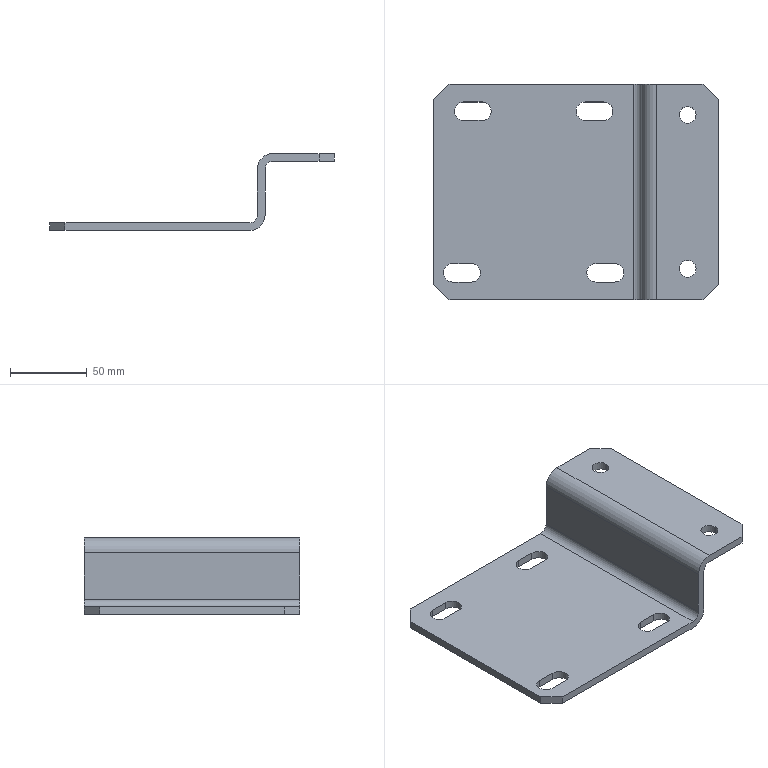Part | STEP file | VD-SYL0380DJ1006_1-8_VD-SYL0380 | 1 solid | 42 faces | box 185 x 140 x 50 mm | volume 149401 mm3 | plane 22 | cylinder 20 | commonest cylinder face diameters 12 x12 11 x4 10 x2 20 x2
STEP:
#1=CARTESIAN_POINT('',(-54.5,-58.5,-40.));
#2=VERTEX_POINT('',#1);
#3=CARTESIAN_POINT('',(-60.5,-52.5,-40.));
#4=VERTEX_POINT('',#3);
#5=CARTESIAN_POINT('',(-54.5,-52.5,-40.));
#6=DIRECTION('',(0.,0.,-1.));
#7=DIRECTION('',(0.,-1.,0.));
#8=AXIS2_PLACEMENT_3D('',#5,#6,#7);
#9=CIRCLE('',#8,6.);
#10=EDGE_CURVE('',#2,#4,#9,.T.);
#11=ORIENTED_EDGE('',*,*,#10,.F.);
#12=CARTESIAN_POINT('',(-54.5,-58.5,-45.));
#13=VERTEX_POINT('',#12);
#14=CARTESIAN_POINT('',(-54.5,-58.5,-40.));
#15=DIRECTION('',(0.,0.,-1.));
#16=VECTOR('',#15,1000.);
#17=LINE('',#14,#16);
#18=EDGE_CURVE('',#2,#13,#17,.T.);
#19=ORIENTED_EDGE('',*,*,#18,.T.);
#20=CARTESIAN_POINT('',(-60.5,-52.5,-45.));
#21=VERTEX_POINT('',#20);
#22=CARTESIAN_POINT('',(-54.5,-52.5,-45.));
#23=DIRECTION('',(0.,0.,1.));
#24=DIRECTION('',(-1.,0.,0.));
#25=AXIS2_PLACEMENT_3D('',#22,#23,#24);
#26=CIRCLE('',#25,6.);
#27=EDGE_CURVE('',#21,#13,#26,.T.);
#28=ORIENTED_EDGE('',*,*,#27,.F.);
#29=CARTESIAN_POINT('',(-60.5,-52.5,-45.));
#30=DIRECTION('',(0.,0.,1.));
#31=VECTOR('',#30,1000.);
#32=LINE('',#29,#31);
#33=EDGE_CURVE('',#21,#4,#32,.T.);
#34=ORIENTED_EDGE('',*,*,#33,.T.);
#35=EDGE_LOOP('',(#11,#19,#28,#34));
#36=FACE_OUTER_BOUND('',#35,.T.);
#37=CARTESIAN_POINT('',(-54.5,-52.5,-42.5));
#38=DIRECTION('',(0.,0.,-1.));
#39=DIRECTION('',(-1.,0.,0.));
#40=AXIS2_PLACEMENT_3D('',#37,#38,#39);
#41=CYLINDRICAL_SURFACE('',#40,6.);
#42=ADVANCED_FACE('',(#36),#41,.F.);
#43=ORIENTED_EDGE('',*,*,#33,.F.);
#44=CARTESIAN_POINT('',(-54.5,-46.5,-45.));
#45=VERTEX_POINT('',#44);
#46=CARTESIAN_POINT('',(-54.5,-52.5,-45.));
#47=DIRECTION('',(0.,0.,1.));
#48=DIRECTION('',(0.,1.,0.));
#49=AXIS2_PLACEMENT_3D('',#46,#47,#48);
#50=CIRCLE('',#49,6.);
#51=EDGE_CURVE('',#45,#21,#50,.T.);
#52=ORIENTED_EDGE('',*,*,#51,.F.);
#53=CARTESIAN_POINT('',(-54.5,-46.5,-40.));
#54=VERTEX_POINT('',#53);
#55=CARTESIAN_POINT('',(-54.5,-46.5,-45.));
#56=DIRECTION('',(0.,0.,1.));
#57=VECTOR('',#56,1000.);
#58=LINE('',#55,#57);
#59=EDGE_CURVE('',#45,#54,#58,.T.);
#60=ORIENTED_EDGE('',*,*,#59,.T.);
#61=CARTESIAN_POINT('',(-54.5,-52.5,-40.));
#62=DIRECTION('',(0.,0.,-1.));
#63=DIRECTION('',(-1.,0.,0.));
#64=AXIS2_PLACEMENT_3D('',#61,#62,#63);
#65=CIRCLE('',#64,6.);
#66=EDGE_CURVE('',#4,#54,#65,.T.);
#67=ORIENTED_EDGE('',*,*,#66,.F.);
#68=EDGE_LOOP('',(#43,#52,#60,#67));
#69=FACE_OUTER_BOUND('',#68,.T.);
#70=CARTESIAN_POINT('',(-54.5,-52.5,-42.5));
#71=DIRECTION('',(0.,0.,-1.));
#72=DIRECTION('',(-1.,0.,0.));
#73=AXIS2_PLACEMENT_3D('',#70,#71,#72);
#74=CYLINDRICAL_SURFACE('',#73,6.);
#75=ADVANCED_FACE('',(#69),#74,.F.);
#76=CARTESIAN_POINT('',(-42.5,-46.5,-45.));
#77=VERTEX_POINT('',#76);
#78=CARTESIAN_POINT('',(-54.5,-46.5,-45.));
#79=DIRECTION('',(1.,0.,0.));
#80=VECTOR('',#79,1000.);
#81=LINE('',#78,#80);
#82=EDGE_CURVE('',#45,#77,#81,.T.);
#83=ORIENTED_EDGE('',*,*,#82,.T.);
#84=CARTESIAN_POINT('',(-42.5,-46.5,-40.));
#85=VERTEX_POINT('',#84);
#86=CARTESIAN_POINT('',(-42.5,-46.5,-40.));
#87=DIRECTION('',(0.,0.,-1.));
#88=VECTOR('',#87,1000.);
#89=LINE('',#86,#88);
#90=EDGE_CURVE('',#85,#77,#89,.T.);
#91=ORIENTED_EDGE('',*,*,#90,.F.);
#92=CARTESIAN_POINT('',(-54.5,-46.5,-40.));
#93=DIRECTION('',(1.,0.,0.));
#94=VECTOR('',#93,1000.);
#95=LINE('',#92,#94);
#96=EDGE_CURVE('',#54,#85,#95,.T.);
#97=ORIENTED_EDGE('',*,*,#96,.F.);
#98=ORIENTED_EDGE('',*,*,#59,.F.);
#99=EDGE_LOOP('',(#83,#91,#97,#98));
#100=FACE_OUTER_BOUND('',#99,.T.);
#101=CARTESIAN_POINT('',(-48.5,-46.5,-42.5));
#102=DIRECTION('',(0.,-1.,0.));
#103=DIRECTION('',(0.,0.,-1.));
#104=AXIS2_PLACEMENT_3D('',#101,#102,#103);
#105=PLANE('',#104);
#106=ADVANCED_FACE('',(#100),#105,.T.);
#107=CARTESIAN_POINT('',(-42.5,-58.5,-40.));
#108=VERTEX_POINT('',#107);
#109=CARTESIAN_POINT('',(-42.5,-52.5,-40.));
#110=DIRECTION('',(0.,0.,-1.));
#111=DIRECTION('',(0.,1.,0.));
#112=AXIS2_PLACEMENT_3D('',#109,#110,#111);
#113=CIRCLE('',#112,6.);
#114=EDGE_CURVE('',#85,#108,#113,.T.);
#115=ORIENTED_EDGE('',*,*,#114,.F.);
#116=ORIENTED_EDGE('',*,*,#90,.T.);
#117=CARTESIAN_POINT('',(-42.5,-58.5,-45.));
#118=VERTEX_POINT('',#117);
#119=CARTESIAN_POINT('',(-42.5,-52.5,-45.));
#120=DIRECTION('',(0.,0.,1.));
#121=DIRECTION('',(1.,0.,0.));
#122=AXIS2_PLACEMENT_3D('',#119,#120,#121);
#123=CIRCLE('',#122,6.);
#124=EDGE_CURVE('',#118,#77,#123,.T.);
#125=ORIENTED_EDGE('',*,*,#124,.F.);
#126=CARTESIAN_POINT('',(-42.5,-58.5,-45.));
#127=DIRECTION('',(0.,0.,1.));
#128=VECTOR('',#127,1000.);
#129=LINE('',#126,#128);
#130=EDGE_CURVE('',#118,#108,#129,.T.);
#131=ORIENTED_EDGE('',*,*,#130,.T.);
#132=EDGE_LOOP('',(#115,#116,#125,#131));
#133=FACE_OUTER_BOUND('',#132,.T.);
#134=CARTESIAN_POINT('',(-42.5,-52.5,-42.5));
#135=DIRECTION('',(0.,0.,-1.));
#136=DIRECTION('',(-1.,0.,0.));
#137=AXIS2_PLACEMENT_3D('',#134,#135,#136);
#138=CYLINDRICAL_SURFACE('',#137,6.);
#139=ADVANCED_FACE('',(#133),#138,.F.);
#140=CARTESIAN_POINT('',(-42.5,-58.5,-45.));
#141=DIRECTION('',(-1.,0.,0.));
#142=VECTOR('',#141,1000.);
#143=LINE('',#140,#142);
#144=EDGE_CURVE('',#118,#13,#143,.T.);
#145=ORIENTED_EDGE('',*,*,#144,.T.);
#146=ORIENTED_EDGE('',*,*,#18,.F.);
#147=CARTESIAN_POINT('',(-42.5,-58.5,-40.));
#148=DIRECTION('',(-1.,0.,0.));
#149=VECTOR('',#148,1000.);
#150=LINE('',#147,#149);
#151=EDGE_CURVE('',#108,#2,#150,.T.);
#152=ORIENTED_EDGE('',*,*,#151,.F.);
#153=ORIENTED_EDGE('',*,*,#130,.F.);
#154=EDGE_LOOP('',(#145,#146,#152,#153));
#155=FACE_OUTER_BOUND('',#154,.T.);
#156=CARTESIAN_POINT('',(-48.5,-58.5,-42.5));
#157=DIRECTION('',(0.,1.,0.));
#158=DIRECTION('',(1.,0.,0.));
#159=AXIS2_PLACEMENT_3D('',#156,#157,#158);
#160=PLANE('',#159);
#161=ADVANCED_FACE('',(#155),#160,.T.);
#162=CARTESIAN_POINT('',(-147.5,-46.5,-45.));
#163=VERTEX_POINT('',#162);
#164=CARTESIAN_POINT('',(-135.5,-46.5,-45.));
#165=VERTEX_POINT('',#164);
#166=CARTESIAN_POINT('',(-147.5,-46.5,-45.));
#167=DIRECTION('',(1.,0.,0.));
#168=VECTOR('',#167,1000.);
#169=LINE('',#166,#168);
#170=EDGE_CURVE('',#163,#165,#169,.T.);
#171=ORIENTED_EDGE('',*,*,#170,.T.);
#172=CARTESIAN_POINT('',(-135.5,-46.5,-40.));
#173=VERTEX_POINT('',#172);
#174=CARTESIAN_POINT('',(-135.5,-46.5,-40.));
#175=DIRECTION('',(0.,0.,-1.));
#176=VECTOR('',#175,1000.);
#177=LINE('',#174,#176);
#178=EDGE_CURVE('',#173,#165,#177,.T.);
#179=ORIENTED_EDGE('',*,*,#178,.F.);
#180=CARTESIAN_POINT('',(-147.5,-46.5,-40.));
#181=VERTEX_POINT('',#180);
#182=CARTESIAN_POINT('',(-147.5,-46.5,-40.));
#183=DIRECTION('',(1.,0.,0.));
#184=VECTOR('',#183,1000.);
#185=LINE('',#182,#184);
#186=EDGE_CURVE('',#181,#173,#185,.T.);
#187=ORIENTED_EDGE('',*,*,#186,.F.);
#188=CARTESIAN_POINT('',(-147.5,-46.5,-45.));
#189=DIRECTION('',(0.,0.,1.));
#190=VECTOR('',#189,1000.);
#191=LINE('',#188,#190);
#192=EDGE_CURVE('',#163,#181,#191,.T.);
#193=ORIENTED_EDGE('',*,*,#192,.F.);
#194=EDGE_LOOP('',(#171,#179,#187,#193));
#195=FACE_OUTER_BOUND('',#194,.T.);
#196=CARTESIAN_POINT('',(-141.5,-46.5,-42.5));
#197=DIRECTION('',(0.,-1.,0.));
#198=DIRECTION('',(0.,0.,-1.));
#199=AXIS2_PLACEMENT_3D('',#196,#197,#198);
#200=PLANE('',#199);
#201=ADVANCED_FACE('',(#195),#200,.T.);
#202=CARTESIAN_POINT('',(-153.5,-52.5,-45.));
#203=VERTEX_POINT('',#202);
#204=CARTESIAN_POINT('',(-153.5,-52.5,-40.));
#205=VERTEX_POINT('',#204);
#206=CARTESIAN_POINT('',(-153.5,-52.5,-45.));
#207=DIRECTION('',(0.,0.,1.));
#208=VECTOR('',#207,1000.);
#209=LINE('',#206,#208);
#210=EDGE_CURVE('',#203,#205,#209,.T.);
#211=ORIENTED_EDGE('',*,*,#210,.F.);
#212=CARTESIAN_POINT('',(-147.5,-52.5,-45.));
#213=DIRECTION('',(0.,0.,1.));
#214=DIRECTION('',(0.,1.,0.));
#215=AXIS2_PLACEMENT_3D('',#212,#213,#214);
#216=CIRCLE('',#215,6.);
#217=EDGE_CURVE('',#163,#203,#216,.T.);
#218=ORIENTED_EDGE('',*,*,#217,.F.);
#219=ORIENTED_EDGE('',*,*,#192,.T.);
#220=CARTESIAN_POINT('',(-147.5,-52.5,-40.));
#221=DIRECTION('',(0.,0.,-1.));
#222=DIRECTION('',(-1.,0.,0.));
#223=AXIS2_PLACEMENT_3D('',#220,#221,#222);
#224=CIRCLE('',#223,6.);
#225=EDGE_CURVE('',#205,#181,#224,.T.);
#226=ORIENTED_EDGE('',*,*,#225,.F.);
#227=EDGE_LOOP('',(#211,#218,#219,#226));
#228=FACE_OUTER_BOUND('',#227,.T.);
#229=CARTESIAN_POINT('',(-147.5,-52.5,-42.5));
#230=DIRECTION('',(0.,0.,-1.));
#231=DIRECTION('',(-1.,0.,0.));
#232=AXIS2_PLACEMENT_3D('',#229,#230,#231);
#233=CYLINDRICAL_SURFACE('',#232,6.);
#234=ADVANCED_FACE('',(#228),#233,.F.);
#235=CARTESIAN_POINT('',(-147.5,-58.5,-40.));
#236=VERTEX_POINT('',#235);
#237=CARTESIAN_POINT('',(-147.5,-52.5,-40.));
#238=DIRECTION('',(0.,0.,-1.));
#239=DIRECTION('',(0.,-1.,0.));
#240=AXIS2_PLACEMENT_3D('',#237,#238,#239);
#241=CIRCLE('',#240,6.);
#242=EDGE_CURVE('',#236,#205,#241,.T.);
#243=ORIENTED_EDGE('',*,*,#242,.F.);
#244=CARTESIAN_POINT('',(-147.5,-58.5,-45.));
#245=VERTEX_POINT('',#244);
#246=CARTESIAN_POINT('',(-147.5,-58.5,-40.));
#247=DIRECTION('',(0.,0.,-1.));
#248=VECTOR('',#247,1000.);
#249=LINE('',#246,#248);
#250=EDGE_CURVE('',#236,#245,#249,.T.);
#251=ORIENTED_EDGE('',*,*,#250,.T.);
#252=CARTESIAN_POINT('',(-147.5,-52.5,-45.));
#253=DIRECTION('',(0.,0.,1.));
#254=DIRECTION('',(-1.,0.,0.));
#255=AXIS2_PLACEMENT_3D('',#252,#253,#254);
#256=CIRCLE('',#255,6.);
#257=EDGE_CURVE('',#203,#245,#256,.T.);
#258=ORIENTED_EDGE('',*,*,#257,.F.);
#259=ORIENTED_EDGE('',*,*,#210,.T.);
#260=EDGE_LOOP('',(#243,#251,#258,#259));
#261=FACE_OUTER_BOUND('',#260,.T.);
#262=CARTESIAN_POINT('',(-147.5,-52.5,-42.5));
#263=DIRECTION('',(0.,0.,-1.));
#264=DIRECTION('',(-1.,0.,0.));
#265=AXIS2_PLACEMENT_3D('',#262,#263,#264);
#266=CYLINDRICAL_SURFACE('',#265,6.);
#267=ADVANCED_FACE('',(#261),#266,.F.);
#268=CARTESIAN_POINT('',(-135.5,-58.5,-45.));
#269=VERTEX_POINT('',#268);
#270=CARTESIAN_POINT('',(-135.5,-58.5,-45.));
#271=DIRECTION('',(-1.,0.,0.));
#272=VECTOR('',#271,1000.);
#273=LINE('',#270,#272);
#274=EDGE_CURVE('',#269,#245,#273,.T.);
#275=ORIENTED_EDGE('',*,*,#274,.T.);
#276=ORIENTED_EDGE('',*,*,#250,.F.);
#277=CARTESIAN_POINT('',(-135.5,-58.5,-40.));
#278=VERTEX_POINT('',#277);
#279=CARTESIAN_POINT('',(-135.5,-58.5,-40.));
#280=DIRECTION('',(-1.,0.,0.));
#281=VECTOR('',#280,1000.);
#282=LINE('',#279,#281);
#283=EDGE_CURVE('',#278,#236,#282,.T.);
#284=ORIENTED_EDGE('',*,*,#283,.F.);
#285=CARTESIAN_POINT('',(-135.5,-58.5,-45.));
#286=DIRECTION('',(0.,0.,1.));
#287=VECTOR('',#286,1000.);
#288=LINE('',#285,#287);
#289=EDGE_CURVE('',#269,#278,#288,.T.);
#290=ORIENTED_EDGE('',*,*,#289,.F.);
#291=EDGE_LOOP('',(#275,#276,#284,#290));
#292=FACE_OUTER_BOUND('',#291,.T.);
#293=CARTESIAN_POINT('',(-141.5,-58.5,-42.5));
#294=DIRECTION('',(0.,1.,0.));
#295=DIRECTION('',(1.,0.,0.));
#296=AXIS2_PLACEMENT_3D('',#293,#294,#295);
#297=PLANE('',#296);
#298=ADVANCED_FACE('',(#292),#297,.T.);
#299=CARTESIAN_POINT('',(-135.5,-52.5,-40.));
#300=DIRECTION('',(0.,0.,-1.));
#301=DIRECTION('',(1.,0.,0.));
#302=AXIS2_PLACEMENT_3D('',#299,#300,#301);
#303=CIRCLE('',#302,6.);
#304=EDGE_CURVE('',#173,#278,#303,.T.);
#305=ORIENTED_EDGE('',*,*,#304,.F.);
#306=ORIENTED_EDGE('',*,*,#178,.T.);
#307=CARTESIAN_POINT('',(-135.5,-52.5,-45.));
#308=DIRECTION('',(0.,0.,1.));
#309=DIRECTION('',(0.,-1.,0.));
#310=AXIS2_PLACEMENT_3D('',#307,#308,#309);
#311=CIRCLE('',#310,6.);
#312=EDGE_CURVE('',#269,#165,#311,.T.);
#313=ORIENTED_EDGE('',*,*,#312,.F.);
#314=ORIENTED_EDGE('',*,*,#289,.T.);
#315=EDGE_LOOP('',(#305,#306,#313,#314));
#316=FACE_OUTER_BOUND('',#315,.T.);
#317=CARTESIAN_POINT('',(-135.5,-52.5,-42.5));
#318=DIRECTION('',(0.,0.,-1.));
#319=DIRECTION('',(-1.,0.,0.));
#320=AXIS2_PLACEMENT_3D('',#317,#318,#319);
#321=CYLINDRICAL_SURFACE('',#320,6.);
#322=ADVANCED_FACE('',(#316),#321,.F.);
#323=CARTESIAN_POINT('',(-61.5,46.5,-40.));
#324=VERTEX_POINT('',#323);
#325=CARTESIAN_POINT('',(-67.5,52.5,-40.));
#326=VERTEX_POINT('',#325);
#327=CARTESIAN_POINT('',(-61.5,52.5,-40.));
#328=DIRECTION('',(0.,0.,-1.));
#329=DIRECTION('',(0.,-1.,0.));
#330=AXIS2_PLACEMENT_3D('',#327,#328,#329);
#331=CIRCLE('',#330,6.);
#332=EDGE_CURVE('',#324,#326,#331,.T.);
#333=ORIENTED_EDGE('',*,*,#332,.F.);
#334=CARTESIAN_POINT('',(-61.5,46.5,-45.));
#335=VERTEX_POINT('',#334);
#336=CARTESIAN_POINT('',(-61.5,46.5,-40.));
#337=DIRECTION('',(0.,0.,-1.));
#338=VECTOR('',#337,1000.);
#339=LINE('',#336,#338);
#340=EDGE_CURVE('',#324,#335,#339,.T.);
#341=ORIENTED_EDGE('',*,*,#340,.T.);
#342=CARTESIAN_POINT('',(-67.5,52.5,-45.));
#343=VERTEX_POINT('',#342);
#344=CARTESIAN_POINT('',(-61.5,52.5,-45.));
#345=DIRECTION('',(0.,0.,1.));
#346=DIRECTION('',(-1.,0.,0.));
#347=AXIS2_PLACEMENT_3D('',#344,#345,#346);
#348=CIRCLE('',#347,6.);
#349=EDGE_CURVE('',#343,#335,#348,.T.);
#350=ORIENTED_EDGE('',*,*,#349,.F.);
#351=CARTESIAN_POINT('',(-67.5,52.5,-45.));
#352=DIRECTION('',(0.,0.,1.));
#353=VECTOR('',#352,1000.);
#354=LINE('',#351,#353);
#355=EDGE_CURVE('',#343,#326,#354,.T.);
#356=ORIENTED_EDGE('',*,*,#355,.T.);
#357=EDGE_LOOP('',(#333,#341,#350,#356));
#358=FACE_OUTER_BOUND('',#357,.T.);
#359=CARTESIAN_POINT('',(-61.5,52.5,-42.5));
#360=DIRECTION('',(0.,0.,-1.));
#361=DIRECTION('',(-1.,0.,0.));
#362=AXIS2_PLACEMENT_3D('',#359,#360,#361);
#363=CYLINDRICAL_SURFACE('',#362,6.);
#364=ADVANCED_FACE('',(#358),#363,.F.);
#365=ORIENTED_EDGE('',*,*,#355,.F.);
#366=CARTESIAN_POINT('',(-61.5,58.5,-45.));
#367=VERTEX_POINT('',#366);
#368=CARTESIAN_POINT('',(-61.5,52.5,-45.));
#369=DIRECTION('',(0.,0.,1.));
#370=DIRECTION('',(0.,1.,0.));
#371=AXIS2_PLACEMENT_3D('',#368,#369,#370);
#372=CIRCLE('',#371,6.);
#373=EDGE_CURVE('',#367,#343,#372,.T.);
#374=ORIENTED_EDGE('',*,*,#373,.F.);
#375=CARTESIAN_POINT('',(-61.5,58.5,-40.));
#376=VERTEX_POINT('',#375);
#377=CARTESIAN_POINT('',(-61.5,58.5,-45.));
#378=DIRECTION('',(0.,0.,1.));
#379=VECTOR('',#378,1000.);
#380=LINE('',#377,#379);
#381=EDGE_CURVE('',#367,#376,#380,.T.);
#382=ORIENTED_EDGE('',*,*,#381,.T.);
#383=CARTESIAN_POINT('',(-61.5,52.5,-40.));
#384=DIRECTION('',(0.,0.,-1.));
#385=DIRECTION('',(-1.,0.,0.));
#386=AXIS2_PLACEMENT_3D('',#383,#384,#385);
#387=CIRCLE('',#386,6.);
#388=EDGE_CURVE('',#326,#376,#387,.T.);
#389=ORIENTED_EDGE('',*,*,#388,.F.);
#390=EDGE_LOOP('',(#365,#374,#382,#389));
#391=FACE_OUTER_BOUND('',#390,.T.);
#392=CARTESIAN_POINT('',(-61.5,52.5,-42.5));
#393=DIRECTION('',(0.,0.,-1.));
#394=DIRECTION('',(-1.,0.,0.));
#395=AXIS2_PLACEMENT_3D('',#392,#393,#394);
#396=CYLINDRICAL_SURFACE('',#395,6.);
#397=ADVANCED_FACE('',(#391),#396,.F.);
#398=CARTESIAN_POINT('',(-49.5,58.5,-45.));
#399=VERTEX_POINT('',#398);
#400=CARTESIAN_POINT('',(-61.5,58.5,-45.));
#401=DIRECTION('',(1.,0.,0.));
#402=VECTOR('',#401,1000.);
#403=LINE('',#400,#402);
#404=EDGE_CURVE('',#367,#399,#403,.T.);
#405=ORIENTED_EDGE('',*,*,#404,.T.);
#406=CARTESIAN_POINT('',(-49.5,58.5,-40.));
#407=VERTEX_POINT('',#406);
#408=CARTESIAN_POINT('',(-49.5,58.5,-40.));
#409=DIRECTION('',(0.,0.,-1.));
#410=VECTOR('',#409,1000.);
#411=LINE('',#408,#410);
#412=EDGE_CURVE('',#407,#399,#411,.T.);
#413=ORIENTED_EDGE('',*,*,#412,.F.);
#414=CARTESIAN_POINT('',(-61.5,58.5,-40.));
#415=DIRECTION('',(1.,0.,0.));
#416=VECTOR('',#415,1000.);
#417=LINE('',#414,#416);
#418=EDGE_CURVE('',#376,#407,#417,.T.);
#419=ORIENTED_EDGE('',*,*,#418,.F.);
#420=ORIENTED_EDGE('',*,*,#381,.F.);
#421=EDGE_LOOP('',(#405,#413,#419,#420));
#422=FACE_OUTER_BOUND('',#421,.T.);
#423=CARTESIAN_POINT('',(-55.5,58.5,-42.5));
#424=DIRECTION('',(0.,-1.,0.));
#425=DIRECTION('',(0.,0.,-1.));
#426=AXIS2_PLACEMENT_3D('',#423,#424,#425);
#427=PLANE('',#426);
#428=ADVANCED_FACE('',(#422),#427,.T.);
#429=CARTESIAN_POINT('',(-49.5,46.5,-40.));
#430=VERTEX_POINT('',#429);
#431=CARTESIAN_POINT('',(-49.5,52.5,-40.));
#432=DIRECTION('',(0.,0.,-1.));
#433=DIRECTION('',(0.,1.,0.));
#434=AXIS2_PLACEMENT_3D('',#431,#432,#433);
#435=CIRCLE('',#434,6.);
#436=EDGE_CURVE('',#407,#430,#435,.T.);
#437=ORIENTED_EDGE('',*,*,#436,.F.);
#438=ORIENTED_EDGE('',*,*,#412,.T.);
#439=CARTESIAN_POINT('',(-49.5,46.5,-45.));
#440=VERTEX_POINT('',#439);
#441=CARTESIAN_POINT('',(-49.5,52.5,-45.));
#442=DIRECTION('',(0.,0.,1.));
#443=DIRECTION('',(1.,0.,0.));
#444=AXIS2_PLACEMENT_3D('',#441,#442,#443);
#445=CIRCLE('',#444,6.);
#446=EDGE_CURVE('',#440,#399,#445,.T.);
#447=ORIENTED_EDGE('',*,*,#446,.F.);
#448=CARTESIAN_POINT('',(-49.5,46.5,-45.));
#449=DIRECTION('',(0.,0.,1.));
#450=VECTOR('',#449,1000.);
#451=LINE('',#448,#450);
#452=EDGE_CURVE('',#440,#430,#451,.T.);
#453=ORIENTED_EDGE('',*,*,#452,.T.);
#454=EDGE_LOOP('',(#437,#438,#447,#453));
#455=FACE_OUTER_BOUND('',#454,.T.);
#456=CARTESIAN_POINT('',(-49.5,52.5,-42.5));
#457=DIRECTION('',(0.,0.,-1.));
#458=DIRECTION('',(-1.,0.,0.));
#459=AXIS2_PLACEMENT_3D('',#456,#457,#458);
#460=CYLINDRICAL_SURFACE('',#459,6.);
#461=ADVANCED_FACE('',(#455),#460,.F.);
#462=CARTESIAN_POINT('',(-49.5,46.5,-45.));
#463=DIRECTION('',(-1.,0.,0.));
#464=VECTOR('',#463,1000.);
#465=LINE('',#462,#464);
#466=EDGE_CURVE('',#440,#335,#465,.T.);
#467=ORIENTED_EDGE('',*,*,#466,.T.);
#468=ORIENTED_EDGE('',*,*,#340,.F.);
#469=CARTESIAN_POINT('',(-49.5,46.5,-40.));
#470=DIRECTION('',(-1.,0.,0.));
#471=VECTOR('',#470,1000.);
#472=LINE('',#469,#471);
#473=EDGE_CURVE('',#430,#324,#472,.T.);
#474=ORIENTED_EDGE('',*,*,#473,.F.);
#475=ORIENTED_EDGE('',*,*,#452,.F.);
#476=EDGE_LOOP('',(#467,#468,#474,#475));
#477=FACE_OUTER_BOUND('',#476,.T.);
#478=CARTESIAN_POINT('',(-55.5,46.5,-42.5));
#479=DIRECTION('',(0.,1.,0.));
#480=DIRECTION('',(1.,0.,0.));
#481=AXIS2_PLACEMENT_3D('',#478,#479,#480);
#482=PLANE('',#481);
#483=ADVANCED_FACE('',(#477),#482,.T.);
#484=CARTESIAN_POINT('',(-140.5,58.5,-45.));
#485=VERTEX_POINT('',#484);
#486=CARTESIAN_POINT('',(-128.5,58.5,-45.));
#487=VERTEX_POINT('',#486);
#488=CARTESIAN_POINT('',(-140.5,58.5,-45.));
#489=DIRECTION('',(1.,0.,0.));
#490=VECTOR('',#489,1000.);
#491=LINE('',#488,#490);
#492=EDGE_CURVE('',#485,#487,#491,.T.);
#493=ORIENTED_EDGE('',*,*,#492,.T.);
#494=CARTESIAN_POINT('',(-128.5,58.5,-40.));
#495=VERTEX_POINT('',#494);
#496=CARTESIAN_POINT('',(-128.5,58.5,-40.));
#497=DIRECTION('',(0.,0.,-1.));
#498=VECTOR('',#497,1000.);
#499=LINE('',#496,#498);
#500=EDGE_CURVE('',#495,#487,#499,.T.);
#501=ORIENTED_EDGE('',*,*,#500,.F.);
#502=CARTESIAN_POINT('',(-140.5,58.5,-40.));
#503=VERTEX_POINT('',#502);
#504=CARTESIAN_POINT('',(-140.5,58.5,-40.));
#505=DIRECTION('',(1.,0.,0.));
#506=VECTOR('',#505,1000.);
#507=LINE('',#504,#506);
#508=EDGE_CURVE('',#503,#495,#507,.T.);
#509=ORIENTED_EDGE('',*,*,#508,.F.);
#510=CARTESIAN_POINT('',(-140.5,58.5,-45.));
#511=DIRECTION('',(0.,0.,1.));
#512=VECTOR('',#511,1000.);
#513=LINE('',#510,#512);
#514=EDGE_CURVE('',#485,#503,#513,.T.);
#515=ORIENTED_EDGE('',*,*,#514,.F.);
#516=EDGE_LOOP('',(#493,#501,#509,#515));
#517=FACE_OUTER_BOUND('',#516,.T.);
#518=CARTESIAN_POINT('',(-134.5,58.5,-42.5));
#519=DIRECTION('',(0.,-1.,0.));
#520=DIRECTION('',(0.,0.,-1.));
#521=AXIS2_PLACEMENT_3D('',#518,#519,#520);
#522=PLANE('',#521);
#523=ADVANCED_FACE('',(#517),#522,.T.);
#524=CARTESIAN_POINT('',(-146.5,52.5,-45.));
#525=VERTEX_POINT('',#524);
#526=CARTESIAN_POINT('',(-146.5,52.5,-40.));
#527=VERTEX_POINT('',#526);
#528=CARTESIAN_POINT('',(-146.5,52.5,-45.));
#529=DIRECTION('',(0.,0.,1.));
#530=VECTOR('',#529,1000.);
#531=LINE('',#528,#530);
#532=EDGE_CURVE('',#525,#527,#531,.T.);
#533=ORIENTED_EDGE('',*,*,#532,.F.);
#534=CARTESIAN_POINT('',(-140.5,52.5,-45.));
#535=DIRECTION('',(0.,0.,1.));
#536=DIRECTION('',(0.,1.,0.));
#537=AXIS2_PLACEMENT_3D('',#534,#535,#536);
#538=CIRCLE('',#537,6.);
#539=EDGE_CURVE('',#485,#525,#538,.T.);
#540=ORIENTED_EDGE('',*,*,#539,.F.);
#541=ORIENTED_EDGE('',*,*,#514,.T.);
#542=CARTESIAN_POINT('',(-140.5,52.5,-40.));
#543=DIRECTION('',(0.,0.,-1.));
#544=DIRECTION('',(-1.,0.,0.));
#545=AXIS2_PLACEMENT_3D('',#542,#543,#544);
#546=CIRCLE('',#545,6.);
#547=EDGE_CURVE('',#527,#503,#546,.T.);
#548=ORIENTED_EDGE('',*,*,#547,.F.);
#549=EDGE_LOOP('',(#533,#540,#541,#548));
#550=FACE_OUTER_BOUND('',#549,.T.);
#551=CARTESIAN_POINT('',(-140.5,52.5,-42.5));
#552=DIRECTION('',(0.,0.,-1.));
#553=DIRECTION('',(-1.,0.,0.));
#554=AXIS2_PLACEMENT_3D('',#551,#552,#553);
#555=CYLINDRICAL_SURFACE('',#554,6.);
#556=ADVANCED_FACE('',(#550),#555,.F.);
#557=CARTESIAN_POINT('',(-140.5,46.5,-40.));
#558=VERTEX_POINT('',#557);
#559=CARTESIAN_POINT('',(-140.5,52.5,-40.));
#560=DIRECTION('',(0.,0.,-1.));
#561=DIRECTION('',(0.,-1.,0.));
#562=AXIS2_PLACEMENT_3D('',#559,#560,#561);
#563=CIRCLE('',#562,6.);
#564=EDGE_CURVE('',#558,#527,#563,.T.);
#565=ORIENTED_EDGE('',*,*,#564,.F.);
#566=CARTESIAN_POINT('',(-140.5,46.5,-45.));
#567=VERTEX_POINT('',#566);
#568=CARTESIAN_POINT('',(-140.5,46.5,-40.));
#569=DIRECTION('',(0.,0.,-1.));
#570=VECTOR('',#569,1000.);
#571=LINE('',#568,#570);
#572=EDGE_CURVE('',#558,#567,#571,.T.);
#573=ORIENTED_EDGE('',*,*,#572,.T.);
#574=CARTESIAN_POINT('',(-140.5,52.5,-45.));
#575=DIRECTION('',(0.,0.,1.));
#576=DIRECTION('',(-1.,0.,0.));
#577=AXIS2_PLACEMENT_3D('',#574,#575,#576);
#578=CIRCLE('',#577,6.);
#579=EDGE_CURVE('',#525,#567,#578,.T.);
#580=ORIENTED_EDGE('',*,*,#579,.F.);
#581=ORIENTED_EDGE('',*,*,#532,.T.);
#582=EDGE_LOOP('',(#565,#573,#580,#581));
#583=FACE_OUTER_BOUND('',#582,.T.);
#584=CARTESIAN_POINT('',(-140.5,52.5,-42.5));
#585=DIRECTION('',(0.,0.,-1.));
#586=DIRECTION('',(-1.,0.,0.));
#587=AXIS2_PLACEMENT_3D('',#584,#585,#586);
#588=CYLINDRICAL_SURFACE('',#587,6.);
#589=ADVANCED_FACE('',(#583),#588,.F.);
#590=CARTESIAN_POINT('',(-128.5,46.5,-45.));
#591=VERTEX_POINT('',#590);
#592=CARTESIAN_POINT('',(-128.5,46.5,-45.));
#593=DIRECTION('',(-1.,0.,0.));
#594=VECTOR('',#593,1000.);
#595=LINE('',#592,#594);
#596=EDGE_CURVE('',#591,#567,#595,.T.);
#597=ORIENTED_EDGE('',*,*,#596,.T.);
#598=ORIENTED_EDGE('',*,*,#572,.F.);
#599=CARTESIAN_POINT('',(-128.5,46.5,-40.));
#600=VERTEX_POINT('',#599);
#601=CARTESIAN_POINT('',(-128.5,46.5,-40.));
#602=DIRECTION('',(-1.,0.,0.));
#603=VECTOR('',#602,1000.);
#604=LINE('',#601,#603);
#605=EDGE_CURVE('',#600,#558,#604,.T.);
#606=ORIENTED_EDGE('',*,*,#605,.F.);
#607=CARTESIAN_POINT('',(-128.5,46.5,-45.));
#608=DIRECTION('',(0.,0.,1.));
#609=VECTOR('',#608,1000.);
#610=LINE('',#607,#609);
#611=EDGE_CURVE('',#591,#600,#610,.T.);
#612=ORIENTED_EDGE('',*,*,#611,.F.);
#613=EDGE_LOOP('',(#597,#598,#606,#612));
#614=FACE_OUTER_BOUND('',#613,.T.);
#615=CARTESIAN_POINT('',(-134.5,46.5,-42.5));
#616=DIRECTION('',(0.,1.,0.));
#617=DIRECTION('',(1.,0.,0.));
#618=AXIS2_PLACEMENT_3D('',#615,#616,#617);
#619=PLANE('',#618);
#620=ADVANCED_FACE('',(#614),#619,.T.);
#621=CARTESIAN_POINT('',(-128.5,52.5,-40.));
#622=DIRECTION('',(0.,0.,-1.));
#623=DIRECTION('',(1.,0.,0.));
#624=AXIS2_PLACEMENT_3D('',#621,#622,#623);
#625=CIRCLE('',#624,6.);
#626=EDGE_CURVE('',#495,#600,#625,.T.);
#627=ORIENTED_EDGE('',*,*,#626,.F.);
#628=ORIENTED_EDGE('',*,*,#500,.T.);
#629=CARTESIAN_POINT('',(-128.5,52.5,-45.));
#630=DIRECTION('',(0.,0.,1.));
#631=DIRECTION('',(0.,-1.,0.));
#632=AXIS2_PLACEMENT_3D('',#629,#630,#631);
#633=CIRCLE('',#632,6.);
#634=EDGE_CURVE('',#591,#487,#633,.T.);
#635=ORIENTED_EDGE('',*,*,#634,.F.);
#636=ORIENTED_EDGE('',*,*,#611,.T.);
#637=EDGE_LOOP('',(#627,#628,#635,#636));
#638=FACE_OUTER_BOUND('',#637,.T.);
#639=CARTESIAN_POINT('',(-128.5,52.5,-42.5));
#640=DIRECTION('',(0.,0.,-1.));
#641=DIRECTION('',(-1.,0.,0.));
#642=AXIS2_PLACEMENT_3D('',#639,#640,#641);
#643=CYLINDRICAL_SURFACE('',#642,6.);
#644=ADVANCED_FACE('',(#638),#643,.F.);
#645=CARTESIAN_POINT('',(-160.,60.,-45.));
#646=VERTEX_POINT('',#645);
#647=CARTESIAN_POINT('',(-150.,70.,-45.));
#648=VERTEX_POINT('',#647);
#649=CARTESIAN_POINT('',(-160.,60.,-45.));
#650=DIRECTION('',(0.7071,0.7071,0.));
#651=VECTOR('',#650,1000.);
#652=LINE('',#649,#651);
#653=EDGE_CURVE('',#646,#648,#652,.T.);
#654=ORIENTED_EDGE('',*,*,#653,.F.);
#655=CARTESIAN_POINT('',(-160.,60.,-40.));
#656=VERTEX_POINT('',#655);
#657=CARTESIAN_POINT('',(-160.,60.,-40.));
#658=DIRECTION('',(0.,0.,-1.));
#659=VECTOR('',#658,1000.);
#660=LINE('',#657,#659);
#661=EDGE_CURVE('',#656,#646,#660,.T.);
#662=ORIENTED_EDGE('',*,*,#661,.F.);
#663=CARTESIAN_POINT('',(-150.,70.,-40.));
#664=VERTEX_POINT('',#663);
#665=CARTESIAN_POINT('',(-150.,70.,-40.));
#666=DIRECTION('',(-0.7071,-0.7071,0.));
#667=VECTOR('',#666,1000.);
#668=LINE('',#665,#667);
#669=EDGE_CURVE('',#664,#656,#668,.T.);
#670=ORIENTED_EDGE('',*,*,#669,.F.);
#671=CARTESIAN_POINT('',(-150.,70.,-45.));
#672=DIRECTION('',(0.,0.,1.));
#673=VECTOR('',#672,1000.);
#674=LINE('',#671,#673);
#675=EDGE_CURVE('',#648,#664,#674,.T.);
#676=ORIENTED_EDGE('',*,*,#675,.F.);
#677=EDGE_LOOP('',(#654,#662,#670,#676));
#678=FACE_OUTER_BOUND('',#677,.T.);
#679=CARTESIAN_POINT('',(-155.,65.,-42.5));
#680=DIRECTION('',(-0.7071,0.7071,0.));
#681=DIRECTION('',(0.,0.,1.));
#682=AXIS2_PLACEMENT_3D('',#679,#680,#681);
#683=PLANE('',#682);
#684=ADVANCED_FACE('',(#678),#683,.T.);
#685=CARTESIAN_POINT('',(-30.,-70.,-45.));
#686=VERTEX_POINT('',#685);
#687=CARTESIAN_POINT('',(-30.,70.,-45.));
#688=VERTEX_POINT('',#687);
#689=CARTESIAN_POINT('',(-30.,-70.,-45.));
#690=DIRECTION('',(0.,1.,0.));
#691=VECTOR('',#690,1000.);
#692=LINE('',#689,#691);
#693=EDGE_CURVE('',#686,#688,#692,.T.);
#694=ORIENTED_EDGE('',*,*,#693,.T.);
#695=CARTESIAN_POINT('',(-20.,70.,-35.));
#696=VERTEX_POINT('',#695);
#697=CARTESIAN_POINT('',(-30.,70.,-35.));
#698=DIRECTION('',(0.,1.,0.));
#699=DIRECTION('',(1.,0.,0.));
#700=AXIS2_PLACEMENT_3D('',#697,#698,#699);
#701=CIRCLE('',#700,10.);
#702=EDGE_CURVE('',#696,#688,#701,.T.);
#703=ORIENTED_EDGE('',*,*,#702,.F.);
#704=CARTESIAN_POINT('',(-20.,-70.,-35.));
#705=VERTEX_POINT('',#704);
#706=CARTESIAN_POINT('',(-20.,70.,-35.));
#707=DIRECTION('',(0.,-1.,0.));
#708=VECTOR('',#707,1000.);
#709=LINE('',#706,#708);
#710=EDGE_CURVE('',#696,#705,#709,.T.);
#711=ORIENTED_EDGE('',*,*,#710,.T.);
#712=CARTESIAN_POINT('',(-30.,-70.,-35.));
#713=DIRECTION('',(0.,-1.,0.));
#714=DIRECTION('',(0.,0.,-1.));
#715=AXIS2_PLACEMENT_3D('',#712,#713,#714);
#716=CIRCLE('',#715,10.);
#717=EDGE_CURVE('',#686,#705,#716,.T.);
#718=ORIENTED_EDGE('',*,*,#717,.F.);
#719=EDGE_LOOP('',(#694,#703,#711,#718));
#720=FACE_OUTER_BOUND('',#719,.T.);
#721=CARTESIAN_POINT('',(-30.,70.,-35.));
#722=DIRECTION('',(0.,-1.,0.));
#723=DIRECTION('',(0.,0.,-1.));
#724=AXIS2_PLACEMENT_3D('',#721,#722,#723);
#725=CYLINDRICAL_SURFACE('',#724,10.);
#726=ADVANCED_FACE('',(#720),#725,.T.);
#727=CARTESIAN_POINT('',(-20.,-70.,-5.));
#728=VERTEX_POINT('',#727);
#729=CARTESIAN_POINT('',(-20.,70.,-5.));
#730=VERTEX_POINT('',#729);
#731=CARTESIAN_POINT('',(-20.,-70.,-5.));
#732=DIRECTION('',(0.,1.,0.));
#733=VECTOR('',#732,1000.);
#734=LINE('',#731,#733);
#735=EDGE_CURVE('',#728,#730,#734,.T.);
#736=ORIENTED_EDGE('',*,*,#735,.F.);
#737=CARTESIAN_POINT('',(-20.,-70.,-5.));
#738=DIRECTION('',(0.,0.,-1.));
#739=VECTOR('',#738,1000.);
#740=LINE('',#737,#739);
#741=EDGE_CURVE('',#728,#705,#740,.T.);
#742=ORIENTED_EDGE('',*,*,#741,.T.);
#743=ORIENTED_EDGE('',*,*,#710,.F.);
#744=CARTESIAN_POINT('',(-20.,70.,-35.));
#745=DIRECTION('',(0.,0.,1.));
#746=VECTOR('',#745,1000.);
#747=LINE('',#744,#746);
#748=EDGE_CURVE('',#696,#730,#747,.T.);
#749=ORIENTED_EDGE('',*,*,#748,.T.);
#750=EDGE_LOOP('',(#736,#742,#743,#749));
#751=FACE_OUTER_BOUND('',#750,.T.);
#752=CARTESIAN_POINT('',(-20.,70.,5.));
#753=DIRECTION('',(-1.,0.,0.));
#754=DIRECTION('',(0.,0.,1.));
#755=AXIS2_PLACEMENT_3D('',#752,#753,#754);
#756=PLANE('',#755);
#757=ADVANCED_FACE('',(#751),#756,.F.);
#758=CARTESIAN_POINT('',(10.5,50.,0.));
#759=VERTEX_POINT('',#758);
#760=CARTESIAN_POINT('',(10.5,50.,5.));
#761=VERTEX_POINT('',#760);
#762=CARTESIAN_POINT('',(10.5,50.,0.));
#763=DIRECTION('',(0.,0.,1.));
#764=VECTOR('',#763,1000.);
#765=LINE('',#762,#764);
#766=EDGE_CURVE('',#759,#761,#765,.T.);
#767=ORIENTED_EDGE('',*,*,#766,.F.);
#768=CARTESIAN_POINT('',(-0.5,50.,0.));
#769=VERTEX_POINT('',#768);
#770=CARTESIAN_POINT('',(5.,50.,0.));
#771=DIRECTION('',(0.,0.,1.));
#772=DIRECTION('',(-1.,0.,0.));
#773=AXIS2_PLACEMENT_3D('',#770,#771,#772);
#774=CIRCLE('',#773,5.5);
#775=EDGE_CURVE('',#769,#759,#774,.T.);
#776=ORIENTED_EDGE('',*,*,#775,.F.);
#777=CARTESIAN_POINT('',(-0.5,50.,5.));
#778=VERTEX_POINT('',#777);
#779=CARTESIAN_POINT('',(-0.5,50.,0.));
#780=DIRECTION('',(0.,0.,1.));
#781=VECTOR('',#780,1000.);
#782=LINE('',#779,#781);
#783=EDGE_CURVE('',#769,#778,#782,.T.);
#784=ORIENTED_EDGE('',*,*,#783,.T.);
#785=CARTESIAN_POINT('',(5.,50.,5.));
#786=DIRECTION('',(0.,0.,-1.));
#787=DIRECTION('',(1.,0.,0.));
#788=AXIS2_PLACEMENT_3D('',#785,#786,#787);
#789=CIRCLE('',#788,5.5);
#790=EDGE_CURVE('',#761,#778,#789,.T.);
#791=ORIENTED_EDGE('',*,*,#790,.F.);
#792=EDGE_LOOP('',(#767,#776,#784,#791));
#793=FACE_OUTER_BOUND('',#792,.T.);
#794=CARTESIAN_POINT('',(5.,50.,2.5));
#795=DIRECTION('',(0.,0.,-1.));
#796=DIRECTION('',(-1.,0.,0.));
#797=AXIS2_PLACEMENT_3D('',#794,#795,#796);
#798=CYLINDRICAL_SURFACE('',#797,5.5);
#799=ADVANCED_FACE('',(#793),#798,.F.);
#800=CARTESIAN_POINT('',(5.,50.,5.));
#801=DIRECTION('',(0.,0.,-1.));
#802=DIRECTION('',(-1.,0.,0.));
#803=AXIS2_PLACEMENT_3D('',#800,#801,#802);
#804=CIRCLE('',#803,5.5);
#805=EDGE_CURVE('',#778,#761,#804,.T.);
#806=ORIENTED_EDGE('',*,*,#805,.F.);
#807=ORIENTED_EDGE('',*,*,#783,.F.);
#808=CARTESIAN_POINT('',(5.,50.,0.));
#809=DIRECTION('',(0.,0.,1.));
#810=DIRECTION('',(1.,0.,0.));
#811=AXIS2_PLACEMENT_3D('',#808,#809,#810);
#812=CIRCLE('',#811,5.5);
#813=EDGE_CURVE('',#759,#769,#812,.T.);
#814=ORIENTED_EDGE('',*,*,#813,.F.);
#815=ORIENTED_EDGE('',*,*,#766,.T.);
#816=EDGE_LOOP('',(#806,#807,#814,#815));
#817=FACE_OUTER_BOUND('',#816,.T.);
#818=CARTESIAN_POINT('',(5.,50.,2.5));
#819=DIRECTION('',(0.,0.,-1.));
#820=DIRECTION('',(-1.,0.,0.));
#821=AXIS2_PLACEMENT_3D('',#818,#819,#820);
#822=CYLINDRICAL_SURFACE('',#821,5.5);
#823=ADVANCED_FACE('',(#817),#822,.F.);
#824=CARTESIAN_POINT('',(10.5,-50.,0.));
#825=VERTEX_POINT('',#824);
#826=CARTESIAN_POINT('',(10.5,-50.,5.));
#827=VERTEX_POINT('',#826);
#828=CARTESIAN_POINT('',(10.5,-50.,0.));
#829=DIRECTION('',(0.,0.,1.));
#830=VECTOR('',#829,1000.);
#831=LINE('',#828,#830);
#832=EDGE_CURVE('',#825,#827,#831,.T.);
#833=ORIENTED_EDGE('',*,*,#832,.F.);
#834=CARTESIAN_POINT('',(-0.5,-50.,0.));
#835=VERTEX_POINT('',#834);
#836=CARTESIAN_POINT('',(5.,-50.,0.));
#837=DIRECTION('',(0.,0.,1.));
#838=DIRECTION('',(-1.,0.,0.));
#839=AXIS2_PLACEMENT_3D('',#836,#837,#838);
#840=CIRCLE('',#839,5.5);
#841=EDGE_CURVE('',#835,#825,#840,.T.);
#842=ORIENTED_EDGE('',*,*,#841,.F.);
#843=CARTESIAN_POINT('',(-0.5,-50.,5.));
#844=VERTEX_POINT('',#843);
#845=CARTESIAN_POINT('',(-0.5,-50.,0.));
#846=DIRECTION('',(0.,0.,1.));
#847=VECTOR('',#846,1000.);
#848=LINE('',#845,#847);
#849=EDGE_CURVE('',#835,#844,#848,.T.);
#850=ORIENTED_EDGE('',*,*,#849,.T.);
#851=CARTESIAN_POINT('',(5.,-50.,5.));
#852=DIRECTION('',(0.,0.,-1.));
#853=DIRECTION('',(1.,0.,0.));
#854=AXIS2_PLACEMENT_3D('',#851,#852,#853);
#855=CIRCLE('',#854,5.5);
#856=EDGE_CURVE('',#827,#844,#855,.T.);
#857=ORIENTED_EDGE('',*,*,#856,.F.);
#858=EDGE_LOOP('',(#833,#842,#850,#857));
#859=FACE_OUTER_BOUND('',#858,.T.);
#860=CARTESIAN_POINT('',(5.,-50.,2.5));
#861=DIRECTION('',(0.,0.,-1.));
#862=DIRECTION('',(-1.,0.,0.));
#863=AXIS2_PLACEMENT_3D('',#860,#861,#862);
#864=CYLINDRICAL_SURFACE('',#863,5.5);
#865=ADVANCED_FACE('',(#859),#864,.F.);
#866=CARTESIAN_POINT('',(5.,-50.,5.));
#867=DIRECTION('',(0.,0.,-1.));
#868=DIRECTION('',(-1.,0.,0.));
#869=AXIS2_PLACEMENT_3D('',#866,#867,#868);
#870=CIRCLE('',#869,5.5);
#871=EDGE_CURVE('',#844,#827,#870,.T.);
#872=ORIENTED_EDGE('',*,*,#871,.F.);
#873=ORIENTED_EDGE('',*,*,#849,.F.);
#874=CARTESIAN_POINT('',(5.,-50.,0.));
#875=DIRECTION('',(0.,0.,1.));
#876=DIRECTION('',(1.,0.,0.));
#877=AXIS2_PLACEMENT_3D('',#874,#875,#876);
#878=CIRCLE('',#877,5.5);
#879=EDGE_CURVE('',#825,#835,#878,.T.);
#880=ORIENTED_EDGE('',*,*,#879,.F.);
#881=ORIENTED_EDGE('',*,*,#832,.T.);
#882=EDGE_LOOP('',(#872,#873,#880,#881));
#883=FACE_OUTER_BOUND('',#882,.T.);
#884=CARTESIAN_POINT('',(5.,-50.,2.5));
#885=DIRECTION('',(0.,0.,-1.));
#886=DIRECTION('',(-1.,0.,0.));
#887=AXIS2_PLACEMENT_3D('',#884,#885,#886);
#888=CYLINDRICAL_SURFACE('',#887,5.5);
#889=ADVANCED_FACE('',(#883),#888,.F.);
#890=CARTESIAN_POINT('',(25.,-60.,0.));
#891=VERTEX_POINT('',#890);
#892=CARTESIAN_POINT('',(15.,-70.,0.));
#893=VERTEX_POINT('',#892);
#894=CARTESIAN_POINT('',(25.,-60.,0.));
#895=DIRECTION('',(-0.7071,-0.7071,0.));
#896=VECTOR('',#895,1000.);
#897=LINE('',#894,#896);
#898=EDGE_CURVE('',#891,#893,#897,.T.);
#899=ORIENTED_EDGE('',*,*,#898,.F.);
#900=CARTESIAN_POINT('',(25.,-60.,5.));
#901=VERTEX_POINT('',#900);
#902=CARTESIAN_POINT('',(25.,-60.,5.));
#903=DIRECTION('',(0.,0.,-1.));
#904=VECTOR('',#903,1000.);
#905=LINE('',#902,#904);
#906=EDGE_CURVE('',#901,#891,#905,.T.);
#907=ORIENTED_EDGE('',*,*,#906,.F.);
#908=CARTESIAN_POINT('',(15.,-70.,5.));
#909=VERTEX_POINT('',#908);
#910=CARTESIAN_POINT('',(15.,-70.,5.));
#911=DIRECTION('',(0.7071,0.7071,0.));
#912=VECTOR('',#911,1000.);
#913=LINE('',#910,#912);
#914=EDGE_CURVE('',#909,#901,#913,.T.);
#915=ORIENTED_EDGE('',*,*,#914,.F.);
#916=CARTESIAN_POINT('',(15.,-70.,0.));
#917=DIRECTION('',(0.,0.,1.));
#918=VECTOR('',#917,1000.);
#919=LINE('',#916,#918);
#920=EDGE_CURVE('',#893,#909,#919,.T.);
#921=ORIENTED_EDGE('',*,*,#920,.F.);
#922=EDGE_LOOP('',(#899,#907,#915,#921));
#923=FACE_OUTER_BOUND('',#922,.T.);
#924=CARTESIAN_POINT('',(20.,-65.,2.5));
#925=DIRECTION('',(0.7071,-0.7071,0.));
#926=DIRECTION('',(0.,0.,-1.));
#927=AXIS2_PLACEMENT_3D('',#924,#925,#926);
#928=PLANE('',#927);
#929=ADVANCED_FACE('',(#923),#928,.T.);
#930=ORIENTED_EDGE('',*,*,#790,.T.);
#931=ORIENTED_EDGE('',*,*,#805,.T.);
#932=EDGE_LOOP('',(#930,#931));
#933=FACE_BOUND('',#932,.T.);
#934=ORIENTED_EDGE('',*,*,#856,.T.);
#935=ORIENTED_EDGE('',*,*,#871,.T.);
#936=EDGE_LOOP('',(#934,#935));
#937=FACE_BOUND('',#936,.T.);
#938=ORIENTED_EDGE('',*,*,#914,.T.);
#939=CARTESIAN_POINT('',(25.,60.,5.));
#940=VERTEX_POINT('',#939);
#941=CARTESIAN_POINT('',(25.,60.,5.));
#942=DIRECTION('',(0.,-1.,0.));
#943=VECTOR('',#942,1000.);
#944=LINE('',#941,#943);
#945=EDGE_CURVE('',#940,#901,#944,.T.);
#946=ORIENTED_EDGE('',*,*,#945,.F.);
#947=CARTESIAN_POINT('',(15.,70.,5.));
#948=VERTEX_POINT('',#947);
#949=CARTESIAN_POINT('',(25.,60.,5.));
#950=DIRECTION('',(-0.7071,0.7071,0.));
#951=VECTOR('',#950,1000.);
#952=LINE('',#949,#951);
#953=EDGE_CURVE('',#940,#948,#952,.T.);
#954=ORIENTED_EDGE('',*,*,#953,.T.);
#955=CARTESIAN_POINT('',(-15.,70.,5.));
#956=VERTEX_POINT('',#955);
#957=CARTESIAN_POINT('',(-15.,70.,5.));
#958=DIRECTION('',(1.,0.,0.));
#959=VECTOR('',#958,1000.);
#960=LINE('',#957,#959);
#961=EDGE_CURVE('',#956,#948,#960,.T.);
#962=ORIENTED_EDGE('',*,*,#961,.F.);
#963=CARTESIAN_POINT('',(-15.,-70.,5.));
#964=VERTEX_POINT('',#963);
#965=CARTESIAN_POINT('',(-15.,-70.,5.));
#966=DIRECTION('',(0.,1.,0.));
#967=VECTOR('',#966,1000.);
#968=LINE('',#965,#967);
#969=EDGE_CURVE('',#964,#956,#968,.T.);
#970=ORIENTED_EDGE('',*,*,#969,.F.);
#971=CARTESIAN_POINT('',(15.,-70.,5.));
#972=DIRECTION('',(-1.,0.,0.));
#973=VECTOR('',#972,1000.);
#974=LINE('',#971,#973);
#975=EDGE_CURVE('',#909,#964,#974,.T.);
#976=ORIENTED_EDGE('',*,*,#975,.F.);
#977=EDGE_LOOP('',(#938,#946,#954,#962,#970,#976));
#978=FACE_OUTER_BOUND('',#977,.T.);
#979=CARTESIAN_POINT('',(0.,0.,5.));
#980=DIRECTION('',(0.,0.,1.));
#981=DIRECTION('',(1.,0.,0.));
#982=AXIS2_PLACEMENT_3D('',#979,#980,#981);
#983=PLANE('',#982);
#984=ADVANCED_FACE('',(#933,#937,#978),#983,.T.);
#985=CARTESIAN_POINT('',(-25.,70.,-5.));
#986=VERTEX_POINT('',#985);
#987=CARTESIAN_POINT('',(-25.,-70.,-5.));
#988=VERTEX_POINT('',#987);
#989=CARTESIAN_POINT('',(-25.,70.,-5.));
#990=DIRECTION('',(0.,-1.,0.));
#991=VECTOR('',#990,1000.);
#992=LINE('',#989,#991);
#993=EDGE_CURVE('',#986,#988,#992,.T.);
#994=ORIENTED_EDGE('',*,*,#993,.T.);
#995=CARTESIAN_POINT('',(-15.,-70.,-5.));
#996=DIRECTION('',(0.,-1.,0.));
#997=DIRECTION('',(0.,0.,1.));
#998=AXIS2_PLACEMENT_3D('',#995,#996,#997);
#999=CIRCLE('',#998,10.);
#1000=EDGE_CURVE('',#964,#988,#999,.T.);
#1001=ORIENTED_EDGE('',*,*,#1000,.F.);
#1002=ORIENTED_EDGE('',*,*,#969,.T.);
#1003=CARTESIAN_POINT('',(-15.,70.,-5.));
#1004=DIRECTION('',(0.,1.,0.));
#1005=DIRECTION('',(-1.,0.,0.));
#1006=AXIS2_PLACEMENT_3D('',#1003,#1004,#1005);
#1007=CIRCLE('',#1006,10.);
#1008=EDGE_CURVE('',#986,#956,#1007,.T.);
#1009=ORIENTED_EDGE('',*,*,#1008,.F.);
#1010=EDGE_LOOP('',(#994,#1001,#1002,#1009));
#1011=FACE_OUTER_BOUND('',#1010,.T.);
#1012=CARTESIAN_POINT('',(-15.,-70.,-5.));
#1013=DIRECTION('',(0.,1.,0.));
#1014=DIRECTION('',(0.,0.,1.));
#1015=AXIS2_PLACEMENT_3D('',#1012,#1013,#1014);
#1016=CYLINDRICAL_SURFACE('',#1015,10.);
#1017=ADVANCED_FACE('',(#1011),#1016,.T.);
#1018=CARTESIAN_POINT('',(-25.,70.,-35.));
#1019=VERTEX_POINT('',#1018);
#1020=CARTESIAN_POINT('',(-25.,70.,-5.));
#1021=DIRECTION('',(0.,0.,-1.));
#1022=VECTOR('',#1021,1000.);
#1023=LINE('',#1020,#1022);
#1024=EDGE_CURVE('',#986,#1019,#1023,.T.);
#1025=ORIENTED_EDGE('',*,*,#1024,.T.);
#1026=CARTESIAN_POINT('',(-25.,-70.,-35.));
#1027=VERTEX_POINT('',#1026);
#1028=CARTESIAN_POINT('',(-25.,-70.,-35.));
#1029=DIRECTION('',(0.,1.,0.));
#1030=VECTOR('',#1029,1000.);
#1031=LINE('',#1028,#1030);
#1032=EDGE_CURVE('',#1027,#1019,#1031,.T.);
#1033=ORIENTED_EDGE('',*,*,#1032,.F.);
#1034=CARTESIAN_POINT('',(-25.,-70.,-35.));
#1035=DIRECTION('',(0.,0.,1.));
#1036=VECTOR('',#1035,1000.);
#1037=LINE('',#1034,#1036);
#1038=EDGE_CURVE('',#1027,#988,#1037,.T.);
#1039=ORIENTED_EDGE('',*,*,#1038,.T.);
#1040=ORIENTED_EDGE('',*,*,#993,.F.);
#1041=EDGE_LOOP('',(#1025,#1033,#1039,#1040));
#1042=FACE_OUTER_BOUND('',#1041,.T.);
#1043=CARTESIAN_POINT('',(-25.,70.,5.));
#1044=DIRECTION('',(-1.,0.,0.));
#1045=DIRECTION('',(0.,0.,1.));
#1046=AXIS2_PLACEMENT_3D('',#1043,#1044,#1045);
#1047=PLANE('',#1046);
#1048=ADVANCED_FACE('',(#1042),#1047,.T.);
#1049=CARTESIAN_POINT('',(-30.,70.,-40.));
#1050=VERTEX_POINT('',#1049);
#1051=CARTESIAN_POINT('',(-30.,70.,-35.));
#1052=DIRECTION('',(0.,-1.,0.));
#1053=DIRECTION('',(0.,0.,-1.));
#1054=AXIS2_PLACEMENT_3D('',#1051,#1052,#1053);
#1055=CIRCLE('',#1054,5.);
#1056=EDGE_CURVE('',#1050,#1019,#1055,.T.);
#1057=ORIENTED_EDGE('',*,*,#1056,.F.);
#1058=CARTESIAN_POINT('',(-30.,-70.,-40.));
#1059=VERTEX_POINT('',#1058);
#1060=CARTESIAN_POINT('',(-30.,70.,-40.));
#1061=DIRECTION('',(0.,-1.,0.));
#1062=VECTOR('',#1061,1000.);
#1063=LINE('',#1060,#1062);
#1064=EDGE_CURVE('',#1050,#1059,#1063,.T.);
#1065=ORIENTED_EDGE('',*,*,#1064,.T.);
#1066=CARTESIAN_POINT('',(-30.,-70.,-35.));
#1067=DIRECTION('',(0.,1.,0.));
#1068=DIRECTION('',(1.,0.,0.));
#1069=AXIS2_PLACEMENT_3D('',#1066,#1067,#1068);
#1070=CIRCLE('',#1069,5.);
#1071=EDGE_CURVE('',#1027,#1059,#1070,.T.);
#1072=ORIENTED_EDGE('',*,*,#1071,.F.);
#1073=ORIENTED_EDGE('',*,*,#1032,.T.);
#1074=EDGE_LOOP('',(#1057,#1065,#1072,#1073));
#1075=FACE_OUTER_BOUND('',#1074,.T.);
#1076=CARTESIAN_POINT('',(-30.,70.,-35.));
#1077=DIRECTION('',(0.,-1.,0.));
#1078=DIRECTION('',(0.,0.,-1.));
#1079=AXIS2_PLACEMENT_3D('',#1076,#1077,#1078);
#1080=CYLINDRICAL_SURFACE('',#1079,5.);
#1081=ADVANCED_FACE('',(#1075),#1080,.F.);
#1082=CARTESIAN_POINT('',(-150.,-70.,-40.));
#1083=VERTEX_POINT('',#1082);
#1084=CARTESIAN_POINT('',(-150.,-70.,-45.));
#1085=VERTEX_POINT('',#1084);
#1086=CARTESIAN_POINT('',(-150.,-70.,-40.));
#1087=DIRECTION('',(0.,0.,-1.));
#1088=VECTOR('',#1087,1000.);
#1089=LINE('',#1086,#1088);
#1090=EDGE_CURVE('',#1083,#1085,#1089,.T.);
#1091=ORIENTED_EDGE('',*,*,#1090,.T.);
#1092=CARTESIAN_POINT('',(-150.,-70.,-45.));
#1093=DIRECTION('',(1.,0.,0.));
#1094=VECTOR('',#1093,1000.);
#1095=LINE('',#1092,#1094);
#1096=EDGE_CURVE('',#1085,#686,#1095,.T.);
#1097=ORIENTED_EDGE('',*,*,#1096,.T.);
#1098=ORIENTED_EDGE('',*,*,#717,.T.);
#1099=ORIENTED_EDGE('',*,*,#741,.F.);
#1100=CARTESIAN_POINT('',(-15.,-70.,0.));
#1101=VERTEX_POINT('',#1100);
#1102=CARTESIAN_POINT('',(-15.,-70.,-5.));
#1103=DIRECTION('',(0.,1.,0.));
#1104=DIRECTION('',(-1.,0.,0.));
#1105=AXIS2_PLACEMENT_3D('',#1102,#1103,#1104);
#1106=CIRCLE('',#1105,5.);
#1107=EDGE_CURVE('',#728,#1101,#1106,.T.);
#1108=ORIENTED_EDGE('',*,*,#1107,.T.);
#1109=CARTESIAN_POINT('',(15.,-70.,0.));
#1110=DIRECTION('',(-1.,0.,0.));
#1111=VECTOR('',#1110,1000.);
#1112=LINE('',#1109,#1111);
#1113=EDGE_CURVE('',#893,#1101,#1112,.T.);
#1114=ORIENTED_EDGE('',*,*,#1113,.F.);
#1115=ORIENTED_EDGE('',*,*,#920,.T.);
#1116=ORIENTED_EDGE('',*,*,#975,.T.);
#1117=ORIENTED_EDGE('',*,*,#1000,.T.);
#1118=ORIENTED_EDGE('',*,*,#1038,.F.);
#1119=ORIENTED_EDGE('',*,*,#1071,.T.);
#1120=CARTESIAN_POINT('',(-150.,-70.,-40.));
#1121=DIRECTION('',(1.,0.,0.));
#1122=VECTOR('',#1121,1000.);
#1123=LINE('',#1120,#1122);
#1124=EDGE_CURVE('',#1083,#1059,#1123,.T.);
#1125=ORIENTED_EDGE('',*,*,#1124,.F.);
#1126=EDGE_LOOP('',(#1091,#1097,#1098,#1099,#1108,#1114,#1115,#1116,#1117,#1118,#1119,#1125));
#1127=FACE_OUTER_BOUND('',#1126,.T.);
#1128=CARTESIAN_POINT('',(-95.,-70.,-42.5));
#1129=DIRECTION('',(0.,-1.,0.));
#1130=DIRECTION('',(0.,0.,-1.));
#1131=AXIS2_PLACEMENT_3D('',#1128,#1129,#1130);
#1132=PLANE('',#1131);
#1133=ADVANCED_FACE('',(#1127),#1132,.T.);
#1134=CARTESIAN_POINT('',(-160.,-60.,-45.));
#1135=VERTEX_POINT('',#1134);
#1136=CARTESIAN_POINT('',(-150.,-70.,-45.));
#1137=DIRECTION('',(-0.7071,0.7071,0.));
#1138=VECTOR('',#1137,1000.);
#1139=LINE('',#1136,#1138);
#1140=EDGE_CURVE('',#1085,#1135,#1139,.T.);
#1141=ORIENTED_EDGE('',*,*,#1140,.F.);
#1142=ORIENTED_EDGE('',*,*,#1090,.F.);
#1143=CARTESIAN_POINT('',(-160.,-60.,-40.));
#1144=VERTEX_POINT('',#1143);
#1145=CARTESIAN_POINT('',(-160.,-60.,-40.));
#1146=DIRECTION('',(0.7071,-0.7071,0.));
#1147=VECTOR('',#1146,1000.);
#1148=LINE('',#1145,#1147);
#1149=EDGE_CURVE('',#1144,#1083,#1148,.T.);
#1150=ORIENTED_EDGE('',*,*,#1149,.F.);
#1151=CARTESIAN_POINT('',(-160.,-60.,-40.));
#1152=DIRECTION('',(0.,0.,-1.));
#1153=VECTOR('',#1152,1000.);
#1154=LINE('',#1151,#1153);
#1155=EDGE_CURVE('',#1144,#1135,#1154,.T.);
#1156=ORIENTED_EDGE('',*,*,#1155,.T.);
#1157=EDGE_LOOP('',(#1141,#1142,#1150,#1156));
#1158=FACE_OUTER_BOUND('',#1157,.T.);
#1159=CARTESIAN_POINT('',(-155.,-65.,-42.5));
#1160=DIRECTION('',(-0.7071,-0.7071,0.));
#1161=DIRECTION('',(-0.7071,0.7071,0.));
#1162=AXIS2_PLACEMENT_3D('',#1159,#1160,#1161);
#1163=PLANE('',#1162);
#1164=ADVANCED_FACE('',(#1158),#1163,.T.);
#1165=ORIENTED_EDGE('',*,*,#10,.T.);
#1166=ORIENTED_EDGE('',*,*,#66,.T.);
#1167=ORIENTED_EDGE('',*,*,#96,.T.);
#1168=ORIENTED_EDGE('',*,*,#114,.T.);
#1169=ORIENTED_EDGE('',*,*,#151,.T.);
#1170=EDGE_LOOP('',(#1165,#1166,#1167,#1168,#1169));
#1171=FACE_BOUND('',#1170,.T.);
#1172=ORIENTED_EDGE('',*,*,#304,.T.);
#1173=ORIENTED_EDGE('',*,*,#283,.T.);
#1174=ORIENTED_EDGE('',*,*,#242,.T.);
#1175=ORIENTED_EDGE('',*,*,#225,.T.);
#1176=ORIENTED_EDGE('',*,*,#186,.T.);
#1177=EDGE_LOOP('',(#1172,#1173,#1174,#1175,#1176));
#1178=FACE_BOUND('',#1177,.T.);
#1179=ORIENTED_EDGE('',*,*,#332,.T.);
#1180=ORIENTED_EDGE('',*,*,#388,.T.);
#1181=ORIENTED_EDGE('',*,*,#418,.T.);
#1182=ORIENTED_EDGE('',*,*,#436,.T.);
#1183=ORIENTED_EDGE('',*,*,#473,.T.);
#1184=EDGE_LOOP('',(#1179,#1180,#1181,#1182,#1183));
#1185=FACE_BOUND('',#1184,.T.);
#1186=ORIENTED_EDGE('',*,*,#626,.T.);
#1187=ORIENTED_EDGE('',*,*,#605,.T.);
#1188=ORIENTED_EDGE('',*,*,#564,.T.);
#1189=ORIENTED_EDGE('',*,*,#547,.T.);
#1190=ORIENTED_EDGE('',*,*,#508,.T.);
#1191=EDGE_LOOP('',(#1186,#1187,#1188,#1189,#1190));
#1192=FACE_BOUND('',#1191,.T.);
#1193=ORIENTED_EDGE('',*,*,#1124,.T.);
#1194=ORIENTED_EDGE('',*,*,#1064,.F.);
#1195=CARTESIAN_POINT('',(-30.,70.,-40.));
#1196=DIRECTION('',(-1.,0.,0.));
#1197=VECTOR('',#1196,1000.);
#1198=LINE('',#1195,#1197);
#1199=EDGE_CURVE('',#1050,#664,#1198,.T.);
#1200=ORIENTED_EDGE('',*,*,#1199,.T.);
#1201=ORIENTED_EDGE('',*,*,#669,.T.);
#1202=CARTESIAN_POINT('',(-160.,60.,-40.));
#1203=DIRECTION('',(0.,-1.,0.));
#1204=VECTOR('',#1203,1000.);
#1205=LINE('',#1202,#1204);
#1206=EDGE_CURVE('',#656,#1144,#1205,.T.);
#1207=ORIENTED_EDGE('',*,*,#1206,.T.);
#1208=ORIENTED_EDGE('',*,*,#1149,.T.);
#1209=EDGE_LOOP('',(#1193,#1194,#1200,#1201,#1207,#1208));
#1210=FACE_OUTER_BOUND('',#1209,.T.);
#1211=CARTESIAN_POINT('',(-20.,-70.,-40.));
#1212=DIRECTION('',(0.,0.,-1.));
#1213=DIRECTION('',(0.,-1.,0.));
#1214=AXIS2_PLACEMENT_3D('',#1211,#1212,#1213);
#1215=PLANE('',#1214);
#1216=ADVANCED_FACE('',(#1171,#1178,#1185,#1192,#1210),#1215,.F.);
#1217=ORIENTED_EDGE('',*,*,#661,.T.);
#1218=CARTESIAN_POINT('',(-160.,60.,-45.));
#1219=DIRECTION('',(0.,-1.,0.));
#1220=VECTOR('',#1219,1000.);
#1221=LINE('',#1218,#1220);
#1222=EDGE_CURVE('',#646,#1135,#1221,.T.);
#1223=ORIENTED_EDGE('',*,*,#1222,.T.);
#1224=ORIENTED_EDGE('',*,*,#1155,.F.);
#1225=ORIENTED_EDGE('',*,*,#1206,.F.);
#1226=EDGE_LOOP('',(#1217,#1223,#1224,#1225));
#1227=FACE_OUTER_BOUND('',#1226,.T.);
#1228=CARTESIAN_POINT('',(-160.,0.,-42.5));
#1229=DIRECTION('',(-1.,0.,0.));
#1230=DIRECTION('',(0.,0.,1.));
#1231=AXIS2_PLACEMENT_3D('',#1228,#1229,#1230);
#1232=PLANE('',#1231);
#1233=ADVANCED_FACE('',(#1227),#1232,.T.);
#1234=ORIENTED_EDGE('',*,*,#217,.T.);
#1235=ORIENTED_EDGE('',*,*,#257,.T.);
#1236=ORIENTED_EDGE('',*,*,#274,.F.);
#1237=ORIENTED_EDGE('',*,*,#312,.T.);
#1238=ORIENTED_EDGE('',*,*,#170,.F.);
#1239=EDGE_LOOP('',(#1234,#1235,#1236,#1237,#1238));
#1240=FACE_BOUND('',#1239,.T.);
#1241=ORIENTED_EDGE('',*,*,#124,.T.);
#1242=ORIENTED_EDGE('',*,*,#82,.F.);
#1243=ORIENTED_EDGE('',*,*,#51,.T.);
#1244=ORIENTED_EDGE('',*,*,#27,.T.);
#1245=ORIENTED_EDGE('',*,*,#144,.F.);
#1246=EDGE_LOOP('',(#1241,#1242,#1243,#1244,#1245));
#1247=FACE_BOUND('',#1246,.T.);
#1248=ORIENTED_EDGE('',*,*,#539,.T.);
#1249=ORIENTED_EDGE('',*,*,#579,.T.);
#1250=ORIENTED_EDGE('',*,*,#596,.F.);
#1251=ORIENTED_EDGE('',*,*,#634,.T.);
#1252=ORIENTED_EDGE('',*,*,#492,.F.);
#1253=EDGE_LOOP('',(#1248,#1249,#1250,#1251,#1252));
#1254=FACE_BOUND('',#1253,.T.);
#1255=ORIENTED_EDGE('',*,*,#446,.T.);
#1256=ORIENTED_EDGE('',*,*,#404,.F.);
#1257=ORIENTED_EDGE('',*,*,#373,.T.);
#1258=ORIENTED_EDGE('',*,*,#349,.T.);
#1259=ORIENTED_EDGE('',*,*,#466,.F.);
#1260=EDGE_LOOP('',(#1255,#1256,#1257,#1258,#1259));
#1261=FACE_BOUND('',#1260,.T.);
#1262=ORIENTED_EDGE('',*,*,#653,.T.);
#1263=CARTESIAN_POINT('',(-30.,70.,-45.));
#1264=DIRECTION('',(-1.,0.,0.));
#1265=VECTOR('',#1264,1000.);
#1266=LINE('',#1263,#1265);
#1267=EDGE_CURVE('',#688,#648,#1266,.T.);
#1268=ORIENTED_EDGE('',*,*,#1267,.F.);
#1269=ORIENTED_EDGE('',*,*,#693,.F.);
#1270=ORIENTED_EDGE('',*,*,#1096,.F.);
#1271=ORIENTED_EDGE('',*,*,#1140,.T.);
#1272=ORIENTED_EDGE('',*,*,#1222,.F.);
#1273=EDGE_LOOP('',(#1262,#1268,#1269,#1270,#1271,#1272));
#1274=FACE_OUTER_BOUND('',#1273,.T.);
#1275=CARTESIAN_POINT('',(-20.,-70.,-45.));
#1276=DIRECTION('',(0.,0.,-1.));
#1277=DIRECTION('',(0.,-1.,0.));
#1278=AXIS2_PLACEMENT_3D('',#1275,#1276,#1277);
#1279=PLANE('',#1278);
#1280=ADVANCED_FACE('',(#1240,#1247,#1254,#1261,#1274),#1279,.T.);
#1281=ORIENTED_EDGE('',*,*,#675,.T.);
#1282=ORIENTED_EDGE('',*,*,#1199,.F.);
#1283=ORIENTED_EDGE('',*,*,#1056,.T.);
#1284=ORIENTED_EDGE('',*,*,#1024,.F.);
#1285=ORIENTED_EDGE('',*,*,#1008,.T.);
#1286=ORIENTED_EDGE('',*,*,#961,.T.);
#1287=CARTESIAN_POINT('',(15.,70.,0.));
#1288=VERTEX_POINT('',#1287);
#1289=CARTESIAN_POINT('',(15.,70.,5.));
#1290=DIRECTION('',(0.,0.,-1.));
#1291=VECTOR('',#1290,1000.);
#1292=LINE('',#1289,#1291);
#1293=EDGE_CURVE('',#948,#1288,#1292,.T.);
#1294=ORIENTED_EDGE('',*,*,#1293,.T.);
#1295=CARTESIAN_POINT('',(-15.,70.,0.));
#1296=VERTEX_POINT('',#1295);
#1297=CARTESIAN_POINT('',(-15.,70.,0.));
#1298=DIRECTION('',(1.,0.,0.));
#1299=VECTOR('',#1298,1000.);
#1300=LINE('',#1297,#1299);
#1301=EDGE_CURVE('',#1296,#1288,#1300,.T.);
#1302=ORIENTED_EDGE('',*,*,#1301,.F.);
#1303=CARTESIAN_POINT('',(-15.,70.,-5.));
#1304=DIRECTION('',(0.,-1.,0.));
#1305=DIRECTION('',(0.,0.,1.));
#1306=AXIS2_PLACEMENT_3D('',#1303,#1304,#1305);
#1307=CIRCLE('',#1306,5.);
#1308=EDGE_CURVE('',#1296,#730,#1307,.T.);
#1309=ORIENTED_EDGE('',*,*,#1308,.T.);
#1310=ORIENTED_EDGE('',*,*,#748,.F.);
#1311=ORIENTED_EDGE('',*,*,#702,.T.);
#1312=ORIENTED_EDGE('',*,*,#1267,.T.);
#1313=EDGE_LOOP('',(#1281,#1282,#1283,#1284,#1285,#1286,#1294,#1302,#1309,#1310,#1311,#1312));
#1314=FACE_OUTER_BOUND('',#1313,.T.);
#1315=CARTESIAN_POINT('',(-95.,70.,-42.5));
#1316=DIRECTION('',(0.,1.,0.));
#1317=DIRECTION('',(1.,0.,0.));
#1318=AXIS2_PLACEMENT_3D('',#1315,#1316,#1317);
#1319=PLANE('',#1318);
#1320=ADVANCED_FACE('',(#1314),#1319,.T.);
#1321=ORIENTED_EDGE('',*,*,#1107,.F.);
#1322=ORIENTED_EDGE('',*,*,#735,.T.);
#1323=ORIENTED_EDGE('',*,*,#1308,.F.);
#1324=CARTESIAN_POINT('',(-15.,70.,0.));
#1325=DIRECTION('',(0.,-1.,0.));
#1326=VECTOR('',#1325,1000.);
#1327=LINE('',#1324,#1326);
#1328=EDGE_CURVE('',#1296,#1101,#1327,.T.);
#1329=ORIENTED_EDGE('',*,*,#1328,.T.);
#1330=EDGE_LOOP('',(#1321,#1322,#1323,#1329));
#1331=FACE_OUTER_BOUND('',#1330,.T.);
#1332=CARTESIAN_POINT('',(-15.,-70.,-5.));
#1333=DIRECTION('',(0.,1.,0.));
#1334=DIRECTION('',(0.,0.,1.));
#1335=AXIS2_PLACEMENT_3D('',#1332,#1333,#1334);
#1336=CYLINDRICAL_SURFACE('',#1335,5.);
#1337=ADVANCED_FACE('',(#1331),#1336,.F.);
#1338=ORIENTED_EDGE('',*,*,#841,.T.);
#1339=ORIENTED_EDGE('',*,*,#879,.T.);
#1340=EDGE_LOOP('',(#1338,#1339));
#1341=FACE_BOUND('',#1340,.T.);
#1342=ORIENTED_EDGE('',*,*,#775,.T.);
#1343=ORIENTED_EDGE('',*,*,#813,.T.);
#1344=EDGE_LOOP('',(#1342,#1343));
#1345=FACE_BOUND('',#1344,.T.);
#1346=ORIENTED_EDGE('',*,*,#1301,.T.);
#1347=CARTESIAN_POINT('',(25.,60.,0.));
#1348=VERTEX_POINT('',#1347);
#1349=CARTESIAN_POINT('',(15.,70.,0.));
#1350=DIRECTION('',(0.7071,-0.7071,0.));
#1351=VECTOR('',#1350,1000.);
#1352=LINE('',#1349,#1351);
#1353=EDGE_CURVE('',#1288,#1348,#1352,.T.);
#1354=ORIENTED_EDGE('',*,*,#1353,.T.);
#1355=CARTESIAN_POINT('',(25.,60.,0.));
#1356=DIRECTION('',(0.,-1.,0.));
#1357=VECTOR('',#1356,1000.);
#1358=LINE('',#1355,#1357);
#1359=EDGE_CURVE('',#1348,#891,#1358,.T.);
#1360=ORIENTED_EDGE('',*,*,#1359,.T.);
#1361=ORIENTED_EDGE('',*,*,#898,.T.);
#1362=ORIENTED_EDGE('',*,*,#1113,.T.);
#1363=ORIENTED_EDGE('',*,*,#1328,.F.);
#1364=EDGE_LOOP('',(#1346,#1354,#1360,#1361,#1362,#1363));
#1365=FACE_OUTER_BOUND('',#1364,.T.);
#1366=CARTESIAN_POINT('',(0.,0.,0.));
#1367=DIRECTION('',(0.,0.,1.));
#1368=DIRECTION('',(1.,0.,0.));
#1369=AXIS2_PLACEMENT_3D('',#1366,#1367,#1368);
#1370=PLANE('',#1369);
#1371=ADVANCED_FACE('',(#1341,#1345,#1365),#1370,.F.);
#1372=ORIENTED_EDGE('',*,*,#945,.T.);
#1373=ORIENTED_EDGE('',*,*,#906,.T.);
#1374=ORIENTED_EDGE('',*,*,#1359,.F.);
#1375=CARTESIAN_POINT('',(25.,60.,0.));
#1376=DIRECTION('',(0.,0.,1.));
#1377=VECTOR('',#1376,1000.);
#1378=LINE('',#1375,#1377);
#1379=EDGE_CURVE('',#1348,#940,#1378,.T.);
#1380=ORIENTED_EDGE('',*,*,#1379,.T.);
#1381=EDGE_LOOP('',(#1372,#1373,#1374,#1380));
#1382=FACE_OUTER_BOUND('',#1381,.T.);
#1383=CARTESIAN_POINT('',(25.,0.,2.5));
#1384=DIRECTION('',(-1.,0.,0.));
#1385=DIRECTION('',(0.,0.,1.));
#1386=AXIS2_PLACEMENT_3D('',#1383,#1384,#1385);
#1387=PLANE('',#1386);
#1388=ADVANCED_FACE('',(#1382),#1387,.F.);
#1389=ORIENTED_EDGE('',*,*,#1353,.F.);
#1390=ORIENTED_EDGE('',*,*,#1293,.F.);
#1391=ORIENTED_EDGE('',*,*,#953,.F.);
#1392=ORIENTED_EDGE('',*,*,#1379,.F.);
#1393=EDGE_LOOP('',(#1389,#1390,#1391,#1392));
#1394=FACE_OUTER_BOUND('',#1393,.T.);
#1395=CARTESIAN_POINT('',(20.,65.,2.5));
#1396=DIRECTION('',(0.7071,0.7071,0.));
#1397=DIRECTION('',(0.,0.,-1.));
#1398=AXIS2_PLACEMENT_3D('',#1395,#1396,#1397);
#1399=PLANE('',#1398);
#1400=ADVANCED_FACE('',(#1394),#1399,.T.);
#1401=CLOSED_SHELL('',(#42,#75,#106,#139,#161,#201,#234,#267,#298,#322,#364,#397,#428,#461,#483,#523,#556,#589,#620,#644,#684,#726,#757,#799,#823,#865,#889,#929,#984,#1017,#1048,#1081,#1133,#1164,#1216,#1233,#1280,#1320,#1337,#1371,#1388,#1400));
#1402=MANIFOLD_SOLID_BREP('',#1401);
#1403=CARTESIAN_POINT('',(0.,0.,0.));
#1404=DIRECTION('',(0.,0.,1.));
#1405=DIRECTION('',(1.,0.,0.));
#1406=AXIS2_PLACEMENT_3D('',#1403,#1404,#1405);
#1407=(LENGTH_UNIT()NAMED_UNIT(*)SI_UNIT(.MILLI.,.METRE.));
#1408=UNCERTAINTY_MEASURE_WITH_UNIT(LENGTH_MEASURE(0.00001),#1407,'','');
#1409=(NAMED_UNIT(*)PLANE_ANGLE_UNIT()SI_UNIT($,.RADIAN.));
#1410=(NAMED_UNIT(*)SI_UNIT($,.STERADIAN.)SOLID_ANGLE_UNIT());
#1411=(GEOMETRIC_REPRESENTATION_CONTEXT(3)GLOBAL_UNCERTAINTY_ASSIGNED_CONTEXT((#1408))GLOBAL_UNIT_ASSIGNED_CONTEXT((#1407,#1409,#1410))REPRESENTATION_CONTEXT('',''));
#1412=ADVANCED_BREP_SHAPE_REPRESENTATION('',(#1402,#1406),#1411);